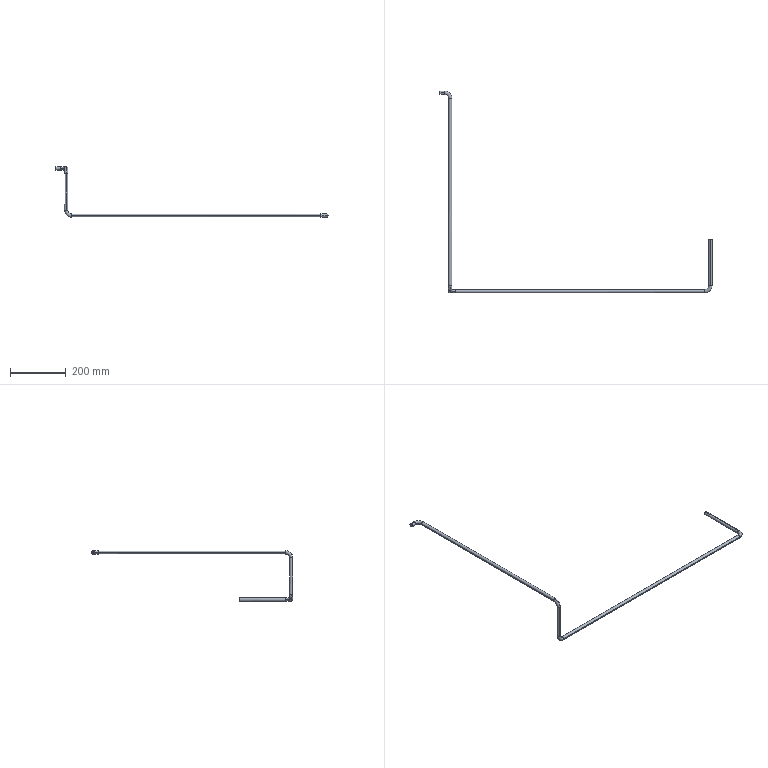Part | SolidWorks | features 3DProfileFeature 2, Sweep 1 | 1 solid | 38 faces | box 973.153 x 721.496 x 180.841 mm | volume 69029 mm3 | cylinder 20 | torus 16 | plane 2 | commonest cylinder face diameters 10 x10 12 x10
STEP:
#1=CARTESIAN_POINT('',(944.95,1782.095,424.913));
#2=VERTEX_POINT('',#1);
#3=CARTESIAN_POINT('',(954.95,1782.095,424.913));
#4=VERTEX_POINT('',#3);
#5=CARTESIAN_POINT('',(949.95,1782.095,424.913));
#6=DIRECTION('',(0.,-1.,0.));
#7=DIRECTION('',(0.,0.,-1.));
#8=AXIS2_PLACEMENT_3D('',#5,#6,#7);
#9=CIRCLE('',#8,5.);
#10=EDGE_CURVE('',#2,#4,#9,.T.);
#11=ORIENTED_EDGE('',*,*,#10,.T.);
#12=CARTESIAN_POINT('',(929.95,1807.095,424.913));
#13=VERTEX_POINT('',#12);
#14=CARTESIAN_POINT('',(929.95,1782.095,424.913));
#15=DIRECTION('',(0.,0.,1.));
#16=DIRECTION('',(1.,0.,0.));
#17=AXIS2_PLACEMENT_3D('',#14,#15,#16);
#18=CIRCLE('',#17,25.);
#19=EDGE_CURVE('',#4,#13,#18,.T.);
#20=ORIENTED_EDGE('',*,*,#19,.T.);
#21=CARTESIAN_POINT('',(929.95,1802.095,419.913));
#22=VERTEX_POINT('',#21);
#23=CARTESIAN_POINT('',(929.95,1802.095,424.913));
#24=DIRECTION('',(1.,0.,0.));
#25=DIRECTION('',(0.,0.,-1.));
#26=AXIS2_PLACEMENT_3D('',#23,#24,#25);
#27=CIRCLE('',#26,5.);
#28=EDGE_CURVE('',#22,#13,#27,.T.);
#29=ORIENTED_EDGE('',*,*,#28,.F.);
#30=CARTESIAN_POINT('',(929.95,1797.095,424.913));
#31=VERTEX_POINT('',#30);
#32=CARTESIAN_POINT('',(929.95,1802.095,424.913));
#33=DIRECTION('',(1.,0.,0.));
#34=DIRECTION('',(0.,0.,-1.));
#35=AXIS2_PLACEMENT_3D('',#32,#33,#34);
#36=CIRCLE('',#35,5.);
#37=EDGE_CURVE('',#31,#22,#36,.T.);
#38=ORIENTED_EDGE('',*,*,#37,.F.);
#39=CARTESIAN_POINT('',(929.95,1782.095,424.913));
#40=DIRECTION('',(0.,0.,1.));
#41=DIRECTION('',(1.,0.,0.));
#42=AXIS2_PLACEMENT_3D('',#39,#40,#41);
#43=CIRCLE('',#42,15.);
#44=EDGE_CURVE('',#2,#31,#43,.T.);
#45=ORIENTED_EDGE('',*,*,#44,.F.);
#46=EDGE_LOOP('',(#11,#20,#29,#38,#45));
#47=FACE_OUTER_BOUND('',#46,.T.);
#48=CARTESIAN_POINT('',(929.95,1782.095,424.913));
#49=DIRECTION('',(0.,0.,1.));
#50=DIRECTION('',(1.,0.,0.));
#51=AXIS2_PLACEMENT_3D('',#48,#49,#50);
#52=TOROIDAL_SURFACE('',#51,20.,5.);
#53=ADVANCED_FACE('',(#47),#52,.F.);
#54=CARTESIAN_POINT('',(949.95,1097.599,404.913));
#55=VERTEX_POINT('',#54);
#56=CARTESIAN_POINT('',(949.95,1087.599,404.913));
#57=VERTEX_POINT('',#56);
#58=CARTESIAN_POINT('',(949.95,1092.599,404.913));
#59=DIRECTION('',(0.,0.,-1.));
#60=DIRECTION('',(0.,1.,0.));
#61=AXIS2_PLACEMENT_3D('',#58,#59,#60);
#62=CIRCLE('',#61,5.);
#63=EDGE_CURVE('',#55,#57,#62,.T.);
#64=ORIENTED_EDGE('',*,*,#63,.T.);
#65=CARTESIAN_POINT('',(949.95,1112.599,429.913));
#66=VERTEX_POINT('',#65);
#67=CARTESIAN_POINT('',(949.95,1112.599,404.913));
#68=DIRECTION('',(-1.,0.,0.));
#69=DIRECTION('',(0.,0.,1.));
#70=AXIS2_PLACEMENT_3D('',#67,#68,#69);
#71=CIRCLE('',#70,25.);
#72=EDGE_CURVE('',#57,#66,#71,.T.);
#73=ORIENTED_EDGE('',*,*,#72,.T.);
#74=CARTESIAN_POINT('',(954.95,1112.599,424.913));
#75=VERTEX_POINT('',#74);
#76=CARTESIAN_POINT('',(949.95,1112.599,424.913));
#77=DIRECTION('',(0.,-1.,0.));
#78=DIRECTION('',(0.,0.,-1.));
#79=AXIS2_PLACEMENT_3D('',#76,#77,#78);
#80=CIRCLE('',#79,5.);
#81=EDGE_CURVE('',#75,#66,#80,.T.);
#82=ORIENTED_EDGE('',*,*,#81,.F.);
#83=CARTESIAN_POINT('',(949.95,1112.599,419.913));
#84=VERTEX_POINT('',#83);
#85=CARTESIAN_POINT('',(949.95,1112.599,424.913));
#86=DIRECTION('',(0.,-1.,0.));
#87=DIRECTION('',(0.,0.,-1.));
#88=AXIS2_PLACEMENT_3D('',#85,#86,#87);
#89=CIRCLE('',#88,5.);
#90=EDGE_CURVE('',#84,#75,#89,.T.);
#91=ORIENTED_EDGE('',*,*,#90,.F.);
#92=CARTESIAN_POINT('',(949.95,1112.599,404.913));
#93=DIRECTION('',(-1.,0.,0.));
#94=DIRECTION('',(0.,0.,1.));
#95=AXIS2_PLACEMENT_3D('',#92,#93,#94);
#96=CIRCLE('',#95,15.);
#97=EDGE_CURVE('',#55,#84,#96,.T.);
#98=ORIENTED_EDGE('',*,*,#97,.F.);
#99=EDGE_LOOP('',(#64,#73,#82,#91,#98));
#100=FACE_OUTER_BOUND('',#99,.T.);
#101=CARTESIAN_POINT('',(949.95,1112.599,404.913));
#102=DIRECTION('',(-1.,0.,0.));
#103=DIRECTION('',(0.,0.,1.));
#104=AXIS2_PLACEMENT_3D('',#101,#102,#103);
#105=TOROIDAL_SURFACE('',#104,20.,5.);
#106=ADVANCED_FACE('',(#100),#105,.F.);
#107=CARTESIAN_POINT('',(969.95,1087.599,256.072));
#108=VERTEX_POINT('',#107);
#109=CARTESIAN_POINT('',(969.95,1092.599,251.072));
#110=VERTEX_POINT('',#109);
#111=CARTESIAN_POINT('',(969.95,1092.599,256.072));
#112=DIRECTION('',(1.,0.,0.));
#113=DIRECTION('',(0.,1.,0.));
#114=AXIS2_PLACEMENT_3D('',#111,#112,#113);
#115=CIRCLE('',#114,5.);
#116=EDGE_CURVE('',#108,#110,#115,.T.);
#117=ORIENTED_EDGE('',*,*,#116,.T.);
#118=CARTESIAN_POINT('',(944.95,1092.599,276.072));
#119=VERTEX_POINT('',#118);
#120=CARTESIAN_POINT('',(969.95,1092.599,276.072));
#121=DIRECTION('',(0.,1.,0.));
#122=DIRECTION('',(-1.,0.,0.));
#123=AXIS2_PLACEMENT_3D('',#120,#121,#122);
#124=CIRCLE('',#123,25.);
#125=EDGE_CURVE('',#110,#119,#124,.T.);
#126=ORIENTED_EDGE('',*,*,#125,.T.);
#127=CARTESIAN_POINT('',(949.95,1087.599,276.072));
#128=VERTEX_POINT('',#127);
#129=CARTESIAN_POINT('',(949.95,1092.599,276.072));
#130=DIRECTION('',(0.,0.,-1.));
#131=DIRECTION('',(0.,1.,0.));
#132=AXIS2_PLACEMENT_3D('',#129,#130,#131);
#133=CIRCLE('',#132,5.);
#134=EDGE_CURVE('',#128,#119,#133,.T.);
#135=ORIENTED_EDGE('',*,*,#134,.F.);
#136=CARTESIAN_POINT('',(954.95,1092.599,276.072));
#137=VERTEX_POINT('',#136);
#138=CARTESIAN_POINT('',(949.95,1092.599,276.072));
#139=DIRECTION('',(0.,0.,-1.));
#140=DIRECTION('',(0.,1.,0.));
#141=AXIS2_PLACEMENT_3D('',#138,#139,#140);
#142=CIRCLE('',#141,5.);
#143=EDGE_CURVE('',#137,#128,#142,.T.);
#144=ORIENTED_EDGE('',*,*,#143,.F.);
#145=CARTESIAN_POINT('',(969.95,1092.599,261.072));
#146=VERTEX_POINT('',#145);
#147=CARTESIAN_POINT('',(969.95,1092.599,276.072));
#148=DIRECTION('',(0.,1.,0.));
#149=DIRECTION('',(-1.,0.,0.));
#150=AXIS2_PLACEMENT_3D('',#147,#148,#149);
#151=CIRCLE('',#150,15.);
#152=EDGE_CURVE('',#146,#137,#151,.T.);
#153=ORIENTED_EDGE('',*,*,#152,.F.);
#154=CARTESIAN_POINT('',(969.95,1092.599,256.072));
#155=DIRECTION('',(1.,0.,0.));
#156=DIRECTION('',(0.,1.,0.));
#157=AXIS2_PLACEMENT_3D('',#154,#155,#156);
#158=CIRCLE('',#157,5.);
#159=EDGE_CURVE('',#146,#108,#158,.T.);
#160=ORIENTED_EDGE('',*,*,#159,.T.);
#161=EDGE_LOOP('',(#117,#126,#135,#144,#153,#160));
#162=FACE_OUTER_BOUND('',#161,.T.);
#163=CARTESIAN_POINT('',(969.95,1092.599,276.072));
#164=DIRECTION('',(0.,1.,0.));
#165=DIRECTION('',(-1.,0.,0.));
#166=AXIS2_PLACEMENT_3D('',#163,#164,#165);
#167=TOROIDAL_SURFACE('',#166,20.,5.);
#168=ADVANCED_FACE('',(#162),#167,.F.);
#169=CARTESIAN_POINT('',(1880.513,1112.599,261.072));
#170=VERTEX_POINT('',#169);
#171=CARTESIAN_POINT('',(1885.513,1112.599,256.072));
#172=VERTEX_POINT('',#171);
#173=CARTESIAN_POINT('',(1880.513,1112.599,256.072));
#174=DIRECTION('',(0.,1.,0.));
#175=DIRECTION('',(-1.,0.,0.));
#176=AXIS2_PLACEMENT_3D('',#173,#174,#175);
#177=CIRCLE('',#176,5.);
#178=EDGE_CURVE('',#170,#172,#177,.T.);
#179=ORIENTED_EDGE('',*,*,#178,.T.);
#180=CARTESIAN_POINT('',(1860.513,1087.599,256.072));
#181=VERTEX_POINT('',#180);
#182=CARTESIAN_POINT('',(1860.513,1112.599,256.072));
#183=DIRECTION('',(0.,0.,-1.));
#184=DIRECTION('',(-1.,0.,0.));
#185=AXIS2_PLACEMENT_3D('',#182,#183,#184);
#186=CIRCLE('',#185,25.);
#187=EDGE_CURVE('',#172,#181,#186,.T.);
#188=ORIENTED_EDGE('',*,*,#187,.T.);
#189=CARTESIAN_POINT('',(1860.513,1097.599,256.072));
#190=VERTEX_POINT('',#189);
#191=CARTESIAN_POINT('',(1860.513,1092.599,256.072));
#192=DIRECTION('',(1.,0.,0.));
#193=DIRECTION('',(0.,1.,0.));
#194=AXIS2_PLACEMENT_3D('',#191,#192,#193);
#195=CIRCLE('',#194,5.);
#196=EDGE_CURVE('',#190,#181,#195,.T.);
#197=ORIENTED_EDGE('',*,*,#196,.F.);
#198=CARTESIAN_POINT('',(1875.513,1112.599,256.072));
#199=VERTEX_POINT('',#198);
#200=CARTESIAN_POINT('',(1860.513,1112.599,256.072));
#201=DIRECTION('',(0.,0.,-1.));
#202=DIRECTION('',(-1.,0.,0.));
#203=AXIS2_PLACEMENT_3D('',#200,#201,#202);
#204=CIRCLE('',#203,15.);
#205=EDGE_CURVE('',#199,#190,#204,.T.);
#206=ORIENTED_EDGE('',*,*,#205,.F.);
#207=CARTESIAN_POINT('',(1880.513,1112.599,256.072));
#208=DIRECTION('',(0.,1.,0.));
#209=DIRECTION('',(-1.,0.,0.));
#210=AXIS2_PLACEMENT_3D('',#207,#208,#209);
#211=CIRCLE('',#210,5.);
#212=EDGE_CURVE('',#199,#170,#211,.T.);
#213=ORIENTED_EDGE('',*,*,#212,.T.);
#214=EDGE_LOOP('',(#179,#188,#197,#206,#213));
#215=FACE_OUTER_BOUND('',#214,.T.);
#216=CARTESIAN_POINT('',(1860.513,1112.599,256.072));
#217=DIRECTION('',(0.,0.,-1.));
#218=DIRECTION('',(-1.,0.,0.));
#219=AXIS2_PLACEMENT_3D('',#216,#217,#218);
#220=TOROIDAL_SURFACE('',#219,20.,5.);
#221=ADVANCED_FACE('',(#215),#220,.F.);
#222=CARTESIAN_POINT('',(955.95,1782.095,424.913));
#223=VERTEX_POINT('',#222);
#224=CARTESIAN_POINT('',(943.95,1782.095,424.913));
#225=VERTEX_POINT('',#224);
#226=CARTESIAN_POINT('',(949.95,1782.095,424.913));
#227=DIRECTION('',(0.,-1.,0.));
#228=DIRECTION('',(-1.,0.,0.));
#229=AXIS2_PLACEMENT_3D('',#226,#227,#228);
#230=CIRCLE('',#229,6.);
#231=EDGE_CURVE('',#223,#225,#230,.T.);
#232=ORIENTED_EDGE('',*,*,#231,.F.);
#233=CARTESIAN_POINT('',(929.95,1808.095,424.913));
#234=VERTEX_POINT('',#233);
#235=CARTESIAN_POINT('',(929.95,1782.095,424.913));
#236=DIRECTION('',(0.,0.,1.));
#237=DIRECTION('',(1.,0.,0.));
#238=AXIS2_PLACEMENT_3D('',#235,#236,#237);
#239=CIRCLE('',#238,26.);
#240=EDGE_CURVE('',#223,#234,#239,.T.);
#241=ORIENTED_EDGE('',*,*,#240,.T.);
#242=CARTESIAN_POINT('',(929.95,1802.095,430.913));
#243=VERTEX_POINT('',#242);
#244=CARTESIAN_POINT('',(929.95,1802.095,424.913));
#245=DIRECTION('',(1.,0.,0.));
#246=DIRECTION('',(0.,1.,0.));
#247=AXIS2_PLACEMENT_3D('',#244,#245,#246);
#248=CIRCLE('',#247,6.);
#249=EDGE_CURVE('',#234,#243,#248,.T.);
#250=ORIENTED_EDGE('',*,*,#249,.T.);
#251=CARTESIAN_POINT('',(929.95,1796.095,424.913));
#252=VERTEX_POINT('',#251);
#253=CARTESIAN_POINT('',(929.95,1802.095,424.913));
#254=DIRECTION('',(1.,0.,0.));
#255=DIRECTION('',(0.,1.,0.));
#256=AXIS2_PLACEMENT_3D('',#253,#254,#255);
#257=CIRCLE('',#256,6.);
#258=EDGE_CURVE('',#243,#252,#257,.T.);
#259=ORIENTED_EDGE('',*,*,#258,.T.);
#260=CARTESIAN_POINT('',(929.95,1782.095,424.913));
#261=DIRECTION('',(0.,0.,1.));
#262=DIRECTION('',(1.,0.,0.));
#263=AXIS2_PLACEMENT_3D('',#260,#261,#262);
#264=CIRCLE('',#263,14.);
#265=EDGE_CURVE('',#225,#252,#264,.T.);
#266=ORIENTED_EDGE('',*,*,#265,.F.);
#267=EDGE_LOOP('',(#232,#241,#250,#259,#266));
#268=FACE_OUTER_BOUND('',#267,.T.);
#269=CARTESIAN_POINT('',(929.95,1782.095,424.913));
#270=DIRECTION('',(0.,0.,1.));
#271=DIRECTION('',(1.,0.,0.));
#272=AXIS2_PLACEMENT_3D('',#269,#270,#271);
#273=TOROIDAL_SURFACE('',#272,20.,6.);
#274=ADVANCED_FACE('',(#268),#273,.T.);
#275=CARTESIAN_POINT('',(949.95,1086.599,404.913));
#276=VERTEX_POINT('',#275);
#277=CARTESIAN_POINT('',(949.95,1098.599,404.913));
#278=VERTEX_POINT('',#277);
#279=CARTESIAN_POINT('',(949.95,1092.599,404.913));
#280=DIRECTION('',(0.,0.,-1.));
#281=DIRECTION('',(0.,-1.,0.));
#282=AXIS2_PLACEMENT_3D('',#279,#280,#281);
#283=CIRCLE('',#282,6.);
#284=EDGE_CURVE('',#276,#278,#283,.T.);
#285=ORIENTED_EDGE('',*,*,#284,.F.);
#286=CARTESIAN_POINT('',(949.95,1112.599,430.913));
#287=VERTEX_POINT('',#286);
#288=CARTESIAN_POINT('',(949.95,1112.599,404.913));
#289=DIRECTION('',(-1.,0.,0.));
#290=DIRECTION('',(0.,0.,1.));
#291=AXIS2_PLACEMENT_3D('',#288,#289,#290);
#292=CIRCLE('',#291,26.);
#293=EDGE_CURVE('',#276,#287,#292,.T.);
#294=ORIENTED_EDGE('',*,*,#293,.T.);
#295=CARTESIAN_POINT('',(943.95,1112.599,424.913));
#296=VERTEX_POINT('',#295);
#297=CARTESIAN_POINT('',(949.95,1112.599,424.913));
#298=DIRECTION('',(0.,-1.,0.));
#299=DIRECTION('',(0.,0.,-1.));
#300=AXIS2_PLACEMENT_3D('',#297,#298,#299);
#301=CIRCLE('',#300,6.);
#302=EDGE_CURVE('',#287,#296,#301,.T.);
#303=ORIENTED_EDGE('',*,*,#302,.T.);
#304=CARTESIAN_POINT('',(949.95,1112.599,418.913));
#305=VERTEX_POINT('',#304);
#306=CARTESIAN_POINT('',(949.95,1112.599,424.913));
#307=DIRECTION('',(0.,-1.,0.));
#308=DIRECTION('',(0.,0.,-1.));
#309=AXIS2_PLACEMENT_3D('',#306,#307,#308);
#310=CIRCLE('',#309,6.);
#311=EDGE_CURVE('',#296,#305,#310,.T.);
#312=ORIENTED_EDGE('',*,*,#311,.T.);
#313=CARTESIAN_POINT('',(949.95,1112.599,404.913));
#314=DIRECTION('',(-1.,0.,0.));
#315=DIRECTION('',(0.,0.,1.));
#316=AXIS2_PLACEMENT_3D('',#313,#314,#315);
#317=CIRCLE('',#316,14.);
#318=EDGE_CURVE('',#278,#305,#317,.T.);
#319=ORIENTED_EDGE('',*,*,#318,.F.);
#320=EDGE_LOOP('',(#285,#294,#303,#312,#319));
#321=FACE_OUTER_BOUND('',#320,.T.);
#322=CARTESIAN_POINT('',(949.95,1112.599,404.913));
#323=DIRECTION('',(-1.,0.,0.));
#324=DIRECTION('',(0.,0.,1.));
#325=AXIS2_PLACEMENT_3D('',#322,#323,#324);
#326=TOROIDAL_SURFACE('',#325,20.,6.);
#327=ADVANCED_FACE('',(#321),#326,.T.);
#328=CARTESIAN_POINT('',(969.95,1092.599,250.072));
#329=VERTEX_POINT('',#328);
#330=CARTESIAN_POINT('',(969.95,1098.599,256.072));
#331=VERTEX_POINT('',#330);
#332=CARTESIAN_POINT('',(969.95,1092.599,256.072));
#333=DIRECTION('',(1.,0.,0.));
#334=DIRECTION('',(0.,-1.,0.));
#335=AXIS2_PLACEMENT_3D('',#332,#333,#334);
#336=CIRCLE('',#335,6.);
#337=EDGE_CURVE('',#329,#331,#336,.T.);
#338=ORIENTED_EDGE('',*,*,#337,.F.);
#339=CARTESIAN_POINT('',(943.95,1092.599,276.072));
#340=VERTEX_POINT('',#339);
#341=CARTESIAN_POINT('',(969.95,1092.599,276.072));
#342=DIRECTION('',(0.,1.,0.));
#343=DIRECTION('',(-1.,0.,0.));
#344=AXIS2_PLACEMENT_3D('',#341,#342,#343);
#345=CIRCLE('',#344,26.);
#346=EDGE_CURVE('',#329,#340,#345,.T.);
#347=ORIENTED_EDGE('',*,*,#346,.T.);
#348=CARTESIAN_POINT('',(949.95,1098.599,276.072));
#349=VERTEX_POINT('',#348);
#350=CARTESIAN_POINT('',(949.95,1092.599,276.072));
#351=DIRECTION('',(0.,0.,-1.));
#352=DIRECTION('',(-1.,0.,0.));
#353=AXIS2_PLACEMENT_3D('',#350,#351,#352);
#354=CIRCLE('',#353,6.);
#355=EDGE_CURVE('',#340,#349,#354,.T.);
#356=ORIENTED_EDGE('',*,*,#355,.T.);
#357=CARTESIAN_POINT('',(955.95,1092.599,276.072));
#358=VERTEX_POINT('',#357);
#359=CARTESIAN_POINT('',(949.95,1092.599,276.072));
#360=DIRECTION('',(0.,0.,-1.));
#361=DIRECTION('',(-1.,0.,0.));
#362=AXIS2_PLACEMENT_3D('',#359,#360,#361);
#363=CIRCLE('',#362,6.);
#364=EDGE_CURVE('',#349,#358,#363,.T.);
#365=ORIENTED_EDGE('',*,*,#364,.T.);
#366=CARTESIAN_POINT('',(969.95,1092.599,262.072));
#367=VERTEX_POINT('',#366);
#368=CARTESIAN_POINT('',(969.95,1092.599,276.072));
#369=DIRECTION('',(0.,1.,0.));
#370=DIRECTION('',(-1.,0.,0.));
#371=AXIS2_PLACEMENT_3D('',#368,#369,#370);
#372=CIRCLE('',#371,14.);
#373=EDGE_CURVE('',#367,#358,#372,.T.);
#374=ORIENTED_EDGE('',*,*,#373,.F.);
#375=CARTESIAN_POINT('',(969.95,1092.599,256.072));
#376=DIRECTION('',(1.,0.,0.));
#377=DIRECTION('',(0.,-1.,0.));
#378=AXIS2_PLACEMENT_3D('',#375,#376,#377);
#379=CIRCLE('',#378,6.);
#380=EDGE_CURVE('',#331,#367,#379,.T.);
#381=ORIENTED_EDGE('',*,*,#380,.F.);
#382=EDGE_LOOP('',(#338,#347,#356,#365,#374,#381));
#383=FACE_OUTER_BOUND('',#382,.T.);
#384=CARTESIAN_POINT('',(969.95,1092.599,276.072));
#385=DIRECTION('',(0.,1.,0.));
#386=DIRECTION('',(-1.,0.,0.));
#387=AXIS2_PLACEMENT_3D('',#384,#385,#386);
#388=TOROIDAL_SURFACE('',#387,20.,6.);
#389=ADVANCED_FACE('',(#383),#388,.T.);
#390=CARTESIAN_POINT('',(1886.513,1112.599,256.072));
#391=VERTEX_POINT('',#390);
#392=CARTESIAN_POINT('',(1880.513,1112.599,250.072));
#393=VERTEX_POINT('',#392);
#394=CARTESIAN_POINT('',(1880.513,1112.599,256.072));
#395=DIRECTION('',(0.,1.,0.));
#396=DIRECTION('',(0.,0.,-1.));
#397=AXIS2_PLACEMENT_3D('',#394,#395,#396);
#398=CIRCLE('',#397,6.);
#399=EDGE_CURVE('',#391,#393,#398,.T.);
#400=ORIENTED_EDGE('',*,*,#399,.F.);
#401=CARTESIAN_POINT('',(1860.513,1086.599,256.072));
#402=VERTEX_POINT('',#401);
#403=CARTESIAN_POINT('',(1860.513,1112.599,256.072));
#404=DIRECTION('',(0.,0.,-1.));
#405=DIRECTION('',(-1.,0.,0.));
#406=AXIS2_PLACEMENT_3D('',#403,#404,#405);
#407=CIRCLE('',#406,26.);
#408=EDGE_CURVE('',#391,#402,#407,.T.);
#409=ORIENTED_EDGE('',*,*,#408,.T.);
#410=CARTESIAN_POINT('',(1860.513,1098.599,256.072));
#411=VERTEX_POINT('',#410);
#412=CARTESIAN_POINT('',(1860.513,1092.599,256.072));
#413=DIRECTION('',(1.,0.,0.));
#414=DIRECTION('',(0.,1.,0.));
#415=AXIS2_PLACEMENT_3D('',#412,#413,#414);
#416=CIRCLE('',#415,6.);
#417=EDGE_CURVE('',#402,#411,#416,.T.);
#418=ORIENTED_EDGE('',*,*,#417,.T.);
#419=CARTESIAN_POINT('',(1874.513,1112.599,256.072));
#420=VERTEX_POINT('',#419);
#421=CARTESIAN_POINT('',(1860.513,1112.599,256.072));
#422=DIRECTION('',(0.,0.,-1.));
#423=DIRECTION('',(-1.,0.,0.));
#424=AXIS2_PLACEMENT_3D('',#421,#422,#423);
#425=CIRCLE('',#424,14.);
#426=EDGE_CURVE('',#420,#411,#425,.T.);
#427=ORIENTED_EDGE('',*,*,#426,.F.);
#428=CARTESIAN_POINT('',(1880.513,1112.599,256.072));
#429=DIRECTION('',(0.,1.,0.));
#430=DIRECTION('',(0.,0.,-1.));
#431=AXIS2_PLACEMENT_3D('',#428,#429,#430);
#432=CIRCLE('',#431,6.);
#433=EDGE_CURVE('',#393,#420,#432,.T.);
#434=ORIENTED_EDGE('',*,*,#433,.F.);
#435=EDGE_LOOP('',(#400,#409,#418,#427,#434));
#436=FACE_OUTER_BOUND('',#435,.T.);
#437=CARTESIAN_POINT('',(1860.513,1112.599,256.072));
#438=DIRECTION('',(0.,0.,-1.));
#439=DIRECTION('',(-1.,0.,0.));
#440=AXIS2_PLACEMENT_3D('',#437,#438,#439);
#441=TOROIDAL_SURFACE('',#440,20.,6.);
#442=ADVANCED_FACE('',(#436),#441,.T.);
#443=CARTESIAN_POINT('',(929.95,1802.095,429.913));
#444=VERTEX_POINT('',#443);
#445=CARTESIAN_POINT('',(929.95,1802.095,424.913));
#446=DIRECTION('',(1.,0.,0.));
#447=DIRECTION('',(0.,0.,-1.));
#448=AXIS2_PLACEMENT_3D('',#445,#446,#447);
#449=CIRCLE('',#448,5.);
#450=EDGE_CURVE('',#444,#31,#449,.T.);
#451=ORIENTED_EDGE('',*,*,#450,.T.);
#452=ORIENTED_EDGE('',*,*,#37,.T.);
#453=CARTESIAN_POINT('',(913.359,1802.095,419.913));
#454=VERTEX_POINT('',#453);
#455=CARTESIAN_POINT('',(929.95,1802.095,419.913));
#456=DIRECTION('',(-1.,0.,0.));
#457=VECTOR('',#456,1000.);
#458=LINE('',#455,#457);
#459=EDGE_CURVE('',#22,#454,#458,.T.);
#460=ORIENTED_EDGE('',*,*,#459,.T.);
#461=CARTESIAN_POINT('',(913.359,1802.095,429.913));
#462=VERTEX_POINT('',#461);
#463=CARTESIAN_POINT('',(913.359,1802.095,424.913));
#464=DIRECTION('',(1.,0.,0.));
#465=DIRECTION('',(0.,0.,-1.));
#466=AXIS2_PLACEMENT_3D('',#463,#464,#465);
#467=CIRCLE('',#466,5.);
#468=EDGE_CURVE('',#462,#454,#467,.T.);
#469=ORIENTED_EDGE('',*,*,#468,.F.);
#470=CARTESIAN_POINT('',(929.95,1802.095,429.913));
#471=DIRECTION('',(-1.,0.,0.));
#472=VECTOR('',#471,1000.);
#473=LINE('',#470,#472);
#474=EDGE_CURVE('',#444,#462,#473,.T.);
#475=ORIENTED_EDGE('',*,*,#474,.F.);
#476=EDGE_LOOP('',(#451,#452,#460,#469,#475));
#477=FACE_OUTER_BOUND('',#476,.T.);
#478=CARTESIAN_POINT('',(929.95,1802.095,424.913));
#479=DIRECTION('',(-1.,0.,0.));
#480=DIRECTION('',(0.,0.,1.));
#481=AXIS2_PLACEMENT_3D('',#478,#479,#480);
#482=CYLINDRICAL_SURFACE('',#481,5.);
#483=ADVANCED_FACE('',(#477),#482,.F.);
#484=CARTESIAN_POINT('',(944.95,1112.599,424.913));
#485=VERTEX_POINT('',#484);
#486=CARTESIAN_POINT('',(949.95,1112.599,424.913));
#487=DIRECTION('',(0.,-1.,0.));
#488=DIRECTION('',(0.,0.,-1.));
#489=AXIS2_PLACEMENT_3D('',#486,#487,#488);
#490=CIRCLE('',#489,5.);
#491=EDGE_CURVE('',#485,#84,#490,.T.);
#492=ORIENTED_EDGE('',*,*,#491,.T.);
#493=ORIENTED_EDGE('',*,*,#90,.T.);
#494=CARTESIAN_POINT('',(954.95,1112.599,424.913));
#495=DIRECTION('',(0.,1.,0.));
#496=VECTOR('',#495,1000.);
#497=LINE('',#494,#496);
#498=EDGE_CURVE('',#75,#4,#497,.T.);
#499=ORIENTED_EDGE('',*,*,#498,.T.);
#500=ORIENTED_EDGE('',*,*,#10,.F.);
#501=CARTESIAN_POINT('',(944.95,1112.599,424.913));
#502=DIRECTION('',(0.,1.,0.));
#503=VECTOR('',#502,1000.);
#504=LINE('',#501,#503);
#505=EDGE_CURVE('',#485,#2,#504,.T.);
#506=ORIENTED_EDGE('',*,*,#505,.F.);
#507=EDGE_LOOP('',(#492,#493,#499,#500,#506));
#508=FACE_OUTER_BOUND('',#507,.T.);
#509=CARTESIAN_POINT('',(949.95,1112.599,424.913));
#510=DIRECTION('',(0.,1.,0.));
#511=DIRECTION('',(-1.,0.,0.));
#512=AXIS2_PLACEMENT_3D('',#509,#510,#511);
#513=CYLINDRICAL_SURFACE('',#512,5.);
#514=ADVANCED_FACE('',(#508),#513,.F.);
#515=ORIENTED_EDGE('',*,*,#134,.T.);
#516=CARTESIAN_POINT('',(949.95,1097.599,276.072));
#517=VERTEX_POINT('',#516);
#518=CARTESIAN_POINT('',(949.95,1092.599,276.072));
#519=DIRECTION('',(0.,0.,-1.));
#520=DIRECTION('',(0.,1.,0.));
#521=AXIS2_PLACEMENT_3D('',#518,#519,#520);
#522=CIRCLE('',#521,5.);
#523=EDGE_CURVE('',#119,#517,#522,.T.);
#524=ORIENTED_EDGE('',*,*,#523,.T.);
#525=CARTESIAN_POINT('',(949.95,1097.599,276.072));
#526=DIRECTION('',(0.,0.,1.));
#527=VECTOR('',#526,1000.);
#528=LINE('',#525,#527);
#529=EDGE_CURVE('',#517,#55,#528,.T.);
#530=ORIENTED_EDGE('',*,*,#529,.T.);
#531=CARTESIAN_POINT('',(949.95,1092.599,404.913));
#532=DIRECTION('',(0.,0.,-1.));
#533=DIRECTION('',(0.,1.,0.));
#534=AXIS2_PLACEMENT_3D('',#531,#532,#533);
#535=CIRCLE('',#534,5.);
#536=EDGE_CURVE('',#57,#55,#535,.T.);
#537=ORIENTED_EDGE('',*,*,#536,.F.);
#538=CARTESIAN_POINT('',(949.95,1087.599,276.072));
#539=DIRECTION('',(0.,0.,1.));
#540=VECTOR('',#539,1000.);
#541=LINE('',#538,#540);
#542=EDGE_CURVE('',#128,#57,#541,.T.);
#543=ORIENTED_EDGE('',*,*,#542,.F.);
#544=EDGE_LOOP('',(#515,#524,#530,#537,#543));
#545=FACE_OUTER_BOUND('',#544,.T.);
#546=CARTESIAN_POINT('',(949.95,1092.599,276.072));
#547=DIRECTION('',(0.,0.,1.));
#548=DIRECTION('',(0.,-1.,0.));
#549=AXIS2_PLACEMENT_3D('',#546,#547,#548);
#550=CYLINDRICAL_SURFACE('',#549,5.);
#551=ADVANCED_FACE('',(#545),#550,.F.);
#552=CARTESIAN_POINT('',(1860.513,1092.599,256.072));
#553=DIRECTION('',(1.,0.,0.));
#554=DIRECTION('',(0.,1.,0.));
#555=AXIS2_PLACEMENT_3D('',#552,#553,#554);
#556=CIRCLE('',#555,5.);
#557=EDGE_CURVE('',#181,#190,#556,.T.);
#558=ORIENTED_EDGE('',*,*,#557,.T.);
#559=CARTESIAN_POINT('',(969.95,1097.599,256.072));
#560=VERTEX_POINT('',#559);
#561=CARTESIAN_POINT('',(1860.513,1097.599,256.072));
#562=DIRECTION('',(-1.,0.,0.));
#563=VECTOR('',#562,1000.);
#564=LINE('',#561,#563);
#565=EDGE_CURVE('',#190,#560,#564,.T.);
#566=ORIENTED_EDGE('',*,*,#565,.T.);
#567=CARTESIAN_POINT('',(969.95,1092.599,256.072));
#568=DIRECTION('',(1.,0.,0.));
#569=DIRECTION('',(0.,1.,0.));
#570=AXIS2_PLACEMENT_3D('',#567,#568,#569);
#571=CIRCLE('',#570,5.);
#572=EDGE_CURVE('',#110,#560,#571,.T.);
#573=ORIENTED_EDGE('',*,*,#572,.F.);
#574=ORIENTED_EDGE('',*,*,#116,.F.);
#575=CARTESIAN_POINT('',(1860.513,1087.599,256.072));
#576=DIRECTION('',(-1.,0.,0.));
#577=VECTOR('',#576,1000.);
#578=LINE('',#575,#577);
#579=EDGE_CURVE('',#181,#108,#578,.T.);
#580=ORIENTED_EDGE('',*,*,#579,.F.);
#581=EDGE_LOOP('',(#558,#566,#573,#574,#580));
#582=FACE_OUTER_BOUND('',#581,.T.);
#583=CARTESIAN_POINT('',(1860.513,1092.599,256.072));
#584=DIRECTION('',(-1.,0.,0.));
#585=DIRECTION('',(0.,-1.,0.));
#586=AXIS2_PLACEMENT_3D('',#583,#584,#585);
#587=CYLINDRICAL_SURFACE('',#586,5.);
#588=ADVANCED_FACE('',(#582),#587,.F.);
#589=CARTESIAN_POINT('',(1880.513,1278.953,251.072));
#590=VERTEX_POINT('',#589);
#591=CARTESIAN_POINT('',(1880.513,1278.953,261.072));
#592=VERTEX_POINT('',#591);
#593=CARTESIAN_POINT('',(1880.513,1278.953,256.072));
#594=DIRECTION('',(0.,1.,0.));
#595=DIRECTION('',(-1.,0.,0.));
#596=AXIS2_PLACEMENT_3D('',#593,#594,#595);
#597=CIRCLE('',#596,5.);
#598=EDGE_CURVE('',#590,#592,#597,.T.);
#599=ORIENTED_EDGE('',*,*,#598,.T.);
#600=CARTESIAN_POINT('',(1880.513,1278.953,261.072));
#601=DIRECTION('',(0.,-1.,0.));
#602=VECTOR('',#601,1000.);
#603=LINE('',#600,#602);
#604=EDGE_CURVE('',#592,#170,#603,.T.);
#605=ORIENTED_EDGE('',*,*,#604,.T.);
#606=ORIENTED_EDGE('',*,*,#212,.F.);
#607=CARTESIAN_POINT('',(1880.513,1112.599,251.072));
#608=VERTEX_POINT('',#607);
#609=CARTESIAN_POINT('',(1880.513,1112.599,256.072));
#610=DIRECTION('',(0.,1.,0.));
#611=DIRECTION('',(-1.,0.,0.));
#612=AXIS2_PLACEMENT_3D('',#609,#610,#611);
#613=CIRCLE('',#612,5.);
#614=EDGE_CURVE('',#608,#199,#613,.T.);
#615=ORIENTED_EDGE('',*,*,#614,.F.);
#616=CARTESIAN_POINT('',(1880.513,1278.953,251.072));
#617=DIRECTION('',(0.,-1.,0.));
#618=VECTOR('',#617,1000.);
#619=LINE('',#616,#618);
#620=EDGE_CURVE('',#590,#608,#619,.T.);
#621=ORIENTED_EDGE('',*,*,#620,.F.);
#622=EDGE_LOOP('',(#599,#605,#606,#615,#621));
#623=FACE_OUTER_BOUND('',#622,.T.);
#624=CARTESIAN_POINT('',(1880.513,1278.953,256.072));
#625=DIRECTION('',(0.,-1.,0.));
#626=DIRECTION('',(0.,0.,-1.));
#627=AXIS2_PLACEMENT_3D('',#624,#625,#626);
#628=CYLINDRICAL_SURFACE('',#627,5.);
#629=ADVANCED_FACE('',(#623),#628,.F.);
#630=CARTESIAN_POINT('',(929.95,1802.095,418.913));
#631=VERTEX_POINT('',#630);
#632=CARTESIAN_POINT('',(929.95,1802.095,424.913));
#633=DIRECTION('',(1.,0.,0.));
#634=DIRECTION('',(0.,1.,0.));
#635=AXIS2_PLACEMENT_3D('',#632,#633,#634);
#636=CIRCLE('',#635,6.);
#637=EDGE_CURVE('',#631,#234,#636,.T.);
#638=ORIENTED_EDGE('',*,*,#637,.F.);
#639=CARTESIAN_POINT('',(913.359,1802.095,418.913));
#640=VERTEX_POINT('',#639);
#641=CARTESIAN_POINT('',(929.95,1802.095,418.913));
#642=DIRECTION('',(-1.,0.,0.));
#643=VECTOR('',#642,1000.);
#644=LINE('',#641,#643);
#645=EDGE_CURVE('',#631,#640,#644,.T.);
#646=ORIENTED_EDGE('',*,*,#645,.T.);
#647=CARTESIAN_POINT('',(913.359,1802.095,430.913));
#648=VERTEX_POINT('',#647);
#649=CARTESIAN_POINT('',(913.359,1802.095,424.913));
#650=DIRECTION('',(1.,0.,0.));
#651=DIRECTION('',(0.,0.,-1.));
#652=AXIS2_PLACEMENT_3D('',#649,#650,#651);
#653=CIRCLE('',#652,6.);
#654=EDGE_CURVE('',#640,#648,#653,.T.);
#655=ORIENTED_EDGE('',*,*,#654,.T.);
#656=CARTESIAN_POINT('',(929.95,1802.095,430.913));
#657=DIRECTION('',(-1.,0.,0.));
#658=VECTOR('',#657,1000.);
#659=LINE('',#656,#658);
#660=EDGE_CURVE('',#243,#648,#659,.T.);
#661=ORIENTED_EDGE('',*,*,#660,.F.);
#662=ORIENTED_EDGE('',*,*,#249,.F.);
#663=EDGE_LOOP('',(#638,#646,#655,#661,#662));
#664=FACE_OUTER_BOUND('',#663,.T.);
#665=CARTESIAN_POINT('',(929.95,1802.095,424.913));
#666=DIRECTION('',(-1.,0.,0.));
#667=DIRECTION('',(0.,0.,1.));
#668=AXIS2_PLACEMENT_3D('',#665,#666,#667);
#669=CYLINDRICAL_SURFACE('',#668,6.);
#670=ADVANCED_FACE('',(#664),#669,.T.);
#671=CARTESIAN_POINT('',(955.95,1112.599,424.913));
#672=VERTEX_POINT('',#671);
#673=CARTESIAN_POINT('',(949.95,1112.599,424.913));
#674=DIRECTION('',(0.,-1.,0.));
#675=DIRECTION('',(0.,0.,-1.));
#676=AXIS2_PLACEMENT_3D('',#673,#674,#675);
#677=CIRCLE('',#676,6.);
#678=EDGE_CURVE('',#672,#287,#677,.T.);
#679=ORIENTED_EDGE('',*,*,#678,.F.);
#680=CARTESIAN_POINT('',(955.95,1112.599,424.913));
#681=DIRECTION('',(0.,1.,0.));
#682=VECTOR('',#681,1000.);
#683=LINE('',#680,#682);
#684=EDGE_CURVE('',#672,#223,#683,.T.);
#685=ORIENTED_EDGE('',*,*,#684,.T.);
#686=ORIENTED_EDGE('',*,*,#231,.T.);
#687=CARTESIAN_POINT('',(943.95,1112.599,424.913));
#688=DIRECTION('',(0.,1.,0.));
#689=VECTOR('',#688,1000.);
#690=LINE('',#687,#689);
#691=EDGE_CURVE('',#296,#225,#690,.T.);
#692=ORIENTED_EDGE('',*,*,#691,.F.);
#693=ORIENTED_EDGE('',*,*,#302,.F.);
#694=EDGE_LOOP('',(#679,#685,#686,#692,#693));
#695=FACE_OUTER_BOUND('',#694,.T.);
#696=CARTESIAN_POINT('',(949.95,1112.599,424.913));
#697=DIRECTION('',(0.,1.,0.));
#698=DIRECTION('',(-1.,0.,0.));
#699=AXIS2_PLACEMENT_3D('',#696,#697,#698);
#700=CYLINDRICAL_SURFACE('',#699,6.);
#701=ADVANCED_FACE('',(#695),#700,.T.);
#702=ORIENTED_EDGE('',*,*,#364,.F.);
#703=CARTESIAN_POINT('',(949.95,1098.599,276.072));
#704=DIRECTION('',(0.,0.,1.));
#705=VECTOR('',#704,1000.);
#706=LINE('',#703,#705);
#707=EDGE_CURVE('',#349,#278,#706,.T.);
#708=ORIENTED_EDGE('',*,*,#707,.T.);
#709=CARTESIAN_POINT('',(949.95,1092.599,404.913));
#710=DIRECTION('',(0.,0.,-1.));
#711=DIRECTION('',(0.,-1.,0.));
#712=AXIS2_PLACEMENT_3D('',#709,#710,#711);
#713=CIRCLE('',#712,6.);
#714=EDGE_CURVE('',#278,#276,#713,.T.);
#715=ORIENTED_EDGE('',*,*,#714,.T.);
#716=CARTESIAN_POINT('',(949.95,1086.599,276.072));
#717=VERTEX_POINT('',#716);
#718=CARTESIAN_POINT('',(949.95,1086.599,276.072));
#719=DIRECTION('',(0.,0.,1.));
#720=VECTOR('',#719,1000.);
#721=LINE('',#718,#720);
#722=EDGE_CURVE('',#717,#276,#721,.T.);
#723=ORIENTED_EDGE('',*,*,#722,.F.);
#724=CARTESIAN_POINT('',(949.95,1092.599,276.072));
#725=DIRECTION('',(0.,0.,-1.));
#726=DIRECTION('',(-1.,0.,0.));
#727=AXIS2_PLACEMENT_3D('',#724,#725,#726);
#728=CIRCLE('',#727,6.);
#729=EDGE_CURVE('',#358,#717,#728,.T.);
#730=ORIENTED_EDGE('',*,*,#729,.F.);
#731=EDGE_LOOP('',(#702,#708,#715,#723,#730));
#732=FACE_OUTER_BOUND('',#731,.T.);
#733=CARTESIAN_POINT('',(949.95,1092.599,276.072));
#734=DIRECTION('',(0.,0.,1.));
#735=DIRECTION('',(0.,-1.,0.));
#736=AXIS2_PLACEMENT_3D('',#733,#734,#735);
#737=CYLINDRICAL_SURFACE('',#736,6.);
#738=ADVANCED_FACE('',(#732),#737,.T.);
#739=CARTESIAN_POINT('',(1860.513,1092.599,256.072));
#740=DIRECTION('',(1.,0.,0.));
#741=DIRECTION('',(0.,1.,0.));
#742=AXIS2_PLACEMENT_3D('',#739,#740,#741);
#743=CIRCLE('',#742,6.);
#744=EDGE_CURVE('',#411,#402,#743,.T.);
#745=ORIENTED_EDGE('',*,*,#744,.F.);
#746=CARTESIAN_POINT('',(1860.513,1098.599,256.072));
#747=DIRECTION('',(-1.,0.,0.));
#748=VECTOR('',#747,1000.);
#749=LINE('',#746,#748);
#750=EDGE_CURVE('',#411,#331,#749,.T.);
#751=ORIENTED_EDGE('',*,*,#750,.T.);
#752=ORIENTED_EDGE('',*,*,#380,.T.);
#753=CARTESIAN_POINT('',(969.95,1086.599,256.072));
#754=VERTEX_POINT('',#753);
#755=CARTESIAN_POINT('',(969.95,1092.599,256.072));
#756=DIRECTION('',(1.,0.,0.));
#757=DIRECTION('',(0.,-1.,0.));
#758=AXIS2_PLACEMENT_3D('',#755,#756,#757);
#759=CIRCLE('',#758,6.);
#760=EDGE_CURVE('',#367,#754,#759,.T.);
#761=ORIENTED_EDGE('',*,*,#760,.T.);
#762=CARTESIAN_POINT('',(1860.513,1086.599,256.072));
#763=DIRECTION('',(-1.,0.,0.));
#764=VECTOR('',#763,1000.);
#765=LINE('',#762,#764);
#766=EDGE_CURVE('',#402,#754,#765,.T.);
#767=ORIENTED_EDGE('',*,*,#766,.F.);
#768=EDGE_LOOP('',(#745,#751,#752,#761,#767));
#769=FACE_OUTER_BOUND('',#768,.T.);
#770=CARTESIAN_POINT('',(1860.513,1092.599,256.072));
#771=DIRECTION('',(-1.,0.,0.));
#772=DIRECTION('',(0.,-1.,0.));
#773=AXIS2_PLACEMENT_3D('',#770,#771,#772);
#774=CYLINDRICAL_SURFACE('',#773,6.);
#775=ADVANCED_FACE('',(#769),#774,.T.);
#776=CARTESIAN_POINT('',(1880.513,1278.953,262.072));
#777=VERTEX_POINT('',#776);
#778=CARTESIAN_POINT('',(1880.513,1278.953,250.072));
#779=VERTEX_POINT('',#778);
#780=CARTESIAN_POINT('',(1880.513,1278.953,256.072));
#781=DIRECTION('',(0.,1.,0.));
#782=DIRECTION('',(0.,0.,1.));
#783=AXIS2_PLACEMENT_3D('',#780,#781,#782);
#784=CIRCLE('',#783,6.);
#785=EDGE_CURVE('',#777,#779,#784,.T.);
#786=ORIENTED_EDGE('',*,*,#785,.F.);
#787=CARTESIAN_POINT('',(1880.513,1112.599,262.072));
#788=VERTEX_POINT('',#787);
#789=CARTESIAN_POINT('',(1880.513,1278.953,262.072));
#790=DIRECTION('',(0.,-1.,0.));
#791=VECTOR('',#790,1000.);
#792=LINE('',#789,#791);
#793=EDGE_CURVE('',#777,#788,#792,.T.);
#794=ORIENTED_EDGE('',*,*,#793,.T.);
#795=CARTESIAN_POINT('',(1880.513,1112.599,256.072));
#796=DIRECTION('',(0.,1.,0.));
#797=DIRECTION('',(0.,0.,-1.));
#798=AXIS2_PLACEMENT_3D('',#795,#796,#797);
#799=CIRCLE('',#798,6.);
#800=EDGE_CURVE('',#788,#391,#799,.T.);
#801=ORIENTED_EDGE('',*,*,#800,.T.);
#802=ORIENTED_EDGE('',*,*,#399,.T.);
#803=CARTESIAN_POINT('',(1880.513,1278.953,250.072));
#804=DIRECTION('',(0.,-1.,0.));
#805=VECTOR('',#804,1000.);
#806=LINE('',#803,#805);
#807=EDGE_CURVE('',#779,#393,#806,.T.);
#808=ORIENTED_EDGE('',*,*,#807,.F.);
#809=EDGE_LOOP('',(#786,#794,#801,#802,#808));
#810=FACE_OUTER_BOUND('',#809,.T.);
#811=CARTESIAN_POINT('',(1880.513,1278.953,256.072));
#812=DIRECTION('',(0.,-1.,0.));
#813=DIRECTION('',(0.,0.,-1.));
#814=AXIS2_PLACEMENT_3D('',#811,#812,#813);
#815=CYLINDRICAL_SURFACE('',#814,6.);
#816=ADVANCED_FACE('',(#810),#815,.T.);
#817=ORIENTED_EDGE('',*,*,#645,.F.);
#818=CARTESIAN_POINT('',(929.95,1802.095,424.913));
#819=DIRECTION('',(1.,0.,0.));
#820=DIRECTION('',(0.,1.,0.));
#821=AXIS2_PLACEMENT_3D('',#818,#819,#820);
#822=CIRCLE('',#821,6.);
#823=EDGE_CURVE('',#252,#631,#822,.T.);
#824=ORIENTED_EDGE('',*,*,#823,.F.);
#825=ORIENTED_EDGE('',*,*,#258,.F.);
#826=ORIENTED_EDGE('',*,*,#660,.T.);
#827=CARTESIAN_POINT('',(913.359,1802.095,424.913));
#828=DIRECTION('',(1.,0.,0.));
#829=DIRECTION('',(0.,0.,-1.));
#830=AXIS2_PLACEMENT_3D('',#827,#828,#829);
#831=CIRCLE('',#830,6.);
#832=EDGE_CURVE('',#648,#640,#831,.T.);
#833=ORIENTED_EDGE('',*,*,#832,.T.);
#834=EDGE_LOOP('',(#817,#824,#825,#826,#833));
#835=FACE_OUTER_BOUND('',#834,.T.);
#836=CARTESIAN_POINT('',(929.95,1802.095,424.913));
#837=DIRECTION('',(-1.,0.,0.));
#838=DIRECTION('',(0.,0.,1.));
#839=AXIS2_PLACEMENT_3D('',#836,#837,#838);
#840=CYLINDRICAL_SURFACE('',#839,6.);
#841=ADVANCED_FACE('',(#835),#840,.T.);
#842=ORIENTED_EDGE('',*,*,#240,.F.);
#843=CARTESIAN_POINT('',(949.95,1782.095,424.913));
#844=DIRECTION('',(0.,-1.,0.));
#845=DIRECTION('',(-1.,0.,0.));
#846=AXIS2_PLACEMENT_3D('',#843,#844,#845);
#847=CIRCLE('',#846,6.);
#848=EDGE_CURVE('',#225,#223,#847,.T.);
#849=ORIENTED_EDGE('',*,*,#848,.F.);
#850=ORIENTED_EDGE('',*,*,#265,.T.);
#851=ORIENTED_EDGE('',*,*,#823,.T.);
#852=ORIENTED_EDGE('',*,*,#637,.T.);
#853=EDGE_LOOP('',(#842,#849,#850,#851,#852));
#854=FACE_OUTER_BOUND('',#853,.T.);
#855=CARTESIAN_POINT('',(929.95,1782.095,424.913));
#856=DIRECTION('',(0.,0.,1.));
#857=DIRECTION('',(1.,0.,0.));
#858=AXIS2_PLACEMENT_3D('',#855,#856,#857);
#859=TOROIDAL_SURFACE('',#858,20.,6.);
#860=ADVANCED_FACE('',(#854),#859,.T.);
#861=ORIENTED_EDGE('',*,*,#684,.F.);
#862=CARTESIAN_POINT('',(949.95,1112.599,424.913));
#863=DIRECTION('',(0.,-1.,0.));
#864=DIRECTION('',(0.,0.,-1.));
#865=AXIS2_PLACEMENT_3D('',#862,#863,#864);
#866=CIRCLE('',#865,6.);
#867=EDGE_CURVE('',#305,#672,#866,.T.);
#868=ORIENTED_EDGE('',*,*,#867,.F.);
#869=ORIENTED_EDGE('',*,*,#311,.F.);
#870=ORIENTED_EDGE('',*,*,#691,.T.);
#871=ORIENTED_EDGE('',*,*,#848,.T.);
#872=EDGE_LOOP('',(#861,#868,#869,#870,#871));
#873=FACE_OUTER_BOUND('',#872,.T.);
#874=CARTESIAN_POINT('',(949.95,1112.599,424.913));
#875=DIRECTION('',(0.,1.,0.));
#876=DIRECTION('',(-1.,0.,0.));
#877=AXIS2_PLACEMENT_3D('',#874,#875,#876);
#878=CYLINDRICAL_SURFACE('',#877,6.);
#879=ADVANCED_FACE('',(#873),#878,.T.);
#880=ORIENTED_EDGE('',*,*,#293,.F.);
#881=ORIENTED_EDGE('',*,*,#714,.F.);
#882=ORIENTED_EDGE('',*,*,#318,.T.);
#883=ORIENTED_EDGE('',*,*,#867,.T.);
#884=ORIENTED_EDGE('',*,*,#678,.T.);
#885=EDGE_LOOP('',(#880,#881,#882,#883,#884));
#886=FACE_OUTER_BOUND('',#885,.T.);
#887=CARTESIAN_POINT('',(949.95,1112.599,404.913));
#888=DIRECTION('',(-1.,0.,0.));
#889=DIRECTION('',(0.,0.,1.));
#890=AXIS2_PLACEMENT_3D('',#887,#888,#889);
#891=TOROIDAL_SURFACE('',#890,20.,6.);
#892=ADVANCED_FACE('',(#886),#891,.T.);
#893=ORIENTED_EDGE('',*,*,#707,.F.);
#894=ORIENTED_EDGE('',*,*,#355,.F.);
#895=CARTESIAN_POINT('',(949.95,1092.599,276.072));
#896=DIRECTION('',(0.,0.,-1.));
#897=DIRECTION('',(-1.,0.,0.));
#898=AXIS2_PLACEMENT_3D('',#895,#896,#897);
#899=CIRCLE('',#898,6.);
#900=EDGE_CURVE('',#717,#340,#899,.T.);
#901=ORIENTED_EDGE('',*,*,#900,.F.);
#902=ORIENTED_EDGE('',*,*,#722,.T.);
#903=ORIENTED_EDGE('',*,*,#284,.T.);
#904=EDGE_LOOP('',(#893,#894,#901,#902,#903));
#905=FACE_OUTER_BOUND('',#904,.T.);
#906=CARTESIAN_POINT('',(949.95,1092.599,276.072));
#907=DIRECTION('',(0.,0.,1.));
#908=DIRECTION('',(0.,-1.,0.));
#909=AXIS2_PLACEMENT_3D('',#906,#907,#908);
#910=CYLINDRICAL_SURFACE('',#909,6.);
#911=ADVANCED_FACE('',(#905),#910,.T.);
#912=ORIENTED_EDGE('',*,*,#346,.F.);
#913=CARTESIAN_POINT('',(969.95,1092.599,256.072));
#914=DIRECTION('',(1.,0.,0.));
#915=DIRECTION('',(0.,-1.,0.));
#916=AXIS2_PLACEMENT_3D('',#913,#914,#915);
#917=CIRCLE('',#916,6.);
#918=EDGE_CURVE('',#754,#329,#917,.T.);
#919=ORIENTED_EDGE('',*,*,#918,.F.);
#920=ORIENTED_EDGE('',*,*,#760,.F.);
#921=ORIENTED_EDGE('',*,*,#373,.T.);
#922=ORIENTED_EDGE('',*,*,#729,.T.);
#923=ORIENTED_EDGE('',*,*,#900,.T.);
#924=EDGE_LOOP('',(#912,#919,#920,#921,#922,#923));
#925=FACE_OUTER_BOUND('',#924,.T.);
#926=CARTESIAN_POINT('',(969.95,1092.599,276.072));
#927=DIRECTION('',(0.,1.,0.));
#928=DIRECTION('',(-1.,0.,0.));
#929=AXIS2_PLACEMENT_3D('',#926,#927,#928);
#930=TOROIDAL_SURFACE('',#929,20.,6.);
#931=ADVANCED_FACE('',(#925),#930,.T.);
#932=ORIENTED_EDGE('',*,*,#750,.F.);
#933=ORIENTED_EDGE('',*,*,#417,.F.);
#934=ORIENTED_EDGE('',*,*,#766,.T.);
#935=ORIENTED_EDGE('',*,*,#918,.T.);
#936=ORIENTED_EDGE('',*,*,#337,.T.);
#937=EDGE_LOOP('',(#932,#933,#934,#935,#936));
#938=FACE_OUTER_BOUND('',#937,.T.);
#939=CARTESIAN_POINT('',(1860.513,1092.599,256.072));
#940=DIRECTION('',(-1.,0.,0.));
#941=DIRECTION('',(0.,-1.,0.));
#942=AXIS2_PLACEMENT_3D('',#939,#940,#941);
#943=CYLINDRICAL_SURFACE('',#942,6.);
#944=ADVANCED_FACE('',(#938),#943,.T.);
#945=ORIENTED_EDGE('',*,*,#408,.F.);
#946=ORIENTED_EDGE('',*,*,#800,.F.);
#947=CARTESIAN_POINT('',(1880.513,1112.599,256.072));
#948=DIRECTION('',(0.,1.,0.));
#949=DIRECTION('',(0.,0.,-1.));
#950=AXIS2_PLACEMENT_3D('',#947,#948,#949);
#951=CIRCLE('',#950,6.);
#952=EDGE_CURVE('',#420,#788,#951,.T.);
#953=ORIENTED_EDGE('',*,*,#952,.F.);
#954=ORIENTED_EDGE('',*,*,#426,.T.);
#955=ORIENTED_EDGE('',*,*,#744,.T.);
#956=EDGE_LOOP('',(#945,#946,#953,#954,#955));
#957=FACE_OUTER_BOUND('',#956,.T.);
#958=CARTESIAN_POINT('',(1860.513,1112.599,256.072));
#959=DIRECTION('',(0.,0.,-1.));
#960=DIRECTION('',(-1.,0.,0.));
#961=AXIS2_PLACEMENT_3D('',#958,#959,#960);
#962=TOROIDAL_SURFACE('',#961,20.,6.);
#963=ADVANCED_FACE('',(#957),#962,.T.);
#964=ORIENTED_EDGE('',*,*,#793,.F.);
#965=CARTESIAN_POINT('',(1880.513,1278.953,256.072));
#966=DIRECTION('',(0.,1.,0.));
#967=DIRECTION('',(0.,0.,1.));
#968=AXIS2_PLACEMENT_3D('',#965,#966,#967);
#969=CIRCLE('',#968,6.);
#970=EDGE_CURVE('',#779,#777,#969,.T.);
#971=ORIENTED_EDGE('',*,*,#970,.F.);
#972=ORIENTED_EDGE('',*,*,#807,.T.);
#973=ORIENTED_EDGE('',*,*,#433,.T.);
#974=ORIENTED_EDGE('',*,*,#952,.T.);
#975=EDGE_LOOP('',(#964,#971,#972,#973,#974));
#976=FACE_OUTER_BOUND('',#975,.T.);
#977=CARTESIAN_POINT('',(1880.513,1278.953,256.072));
#978=DIRECTION('',(0.,-1.,0.));
#979=DIRECTION('',(0.,0.,-1.));
#980=AXIS2_PLACEMENT_3D('',#977,#978,#979);
#981=CYLINDRICAL_SURFACE('',#980,6.);
#982=ADVANCED_FACE('',(#976),#981,.T.);
#983=ORIENTED_EDGE('',*,*,#468,.T.);
#984=CARTESIAN_POINT('',(913.359,1802.095,424.913));
#985=DIRECTION('',(1.,0.,0.));
#986=DIRECTION('',(0.,0.,-1.));
#987=AXIS2_PLACEMENT_3D('',#984,#985,#986);
#988=CIRCLE('',#987,5.);
#989=EDGE_CURVE('',#454,#462,#988,.T.);
#990=ORIENTED_EDGE('',*,*,#989,.T.);
#991=EDGE_LOOP('',(#983,#990));
#992=FACE_BOUND('',#991,.T.);
#993=ORIENTED_EDGE('',*,*,#832,.F.);
#994=ORIENTED_EDGE('',*,*,#654,.F.);
#995=EDGE_LOOP('',(#993,#994));
#996=FACE_OUTER_BOUND('',#995,.T.);
#997=CARTESIAN_POINT('',(913.359,1802.095,424.913));
#998=DIRECTION('',(1.,0.,0.));
#999=DIRECTION('',(0.,0.,-1.));
#1000=AXIS2_PLACEMENT_3D('',#997,#998,#999);
#1001=PLANE('',#1000);
#1002=ADVANCED_FACE('',(#992,#996),#1001,.F.);
#1003=ORIENTED_EDGE('',*,*,#598,.F.);
#1004=CARTESIAN_POINT('',(1880.513,1278.953,256.072));
#1005=DIRECTION('',(0.,1.,0.));
#1006=DIRECTION('',(-1.,0.,0.));
#1007=AXIS2_PLACEMENT_3D('',#1004,#1005,#1006);
#1008=CIRCLE('',#1007,5.);
#1009=EDGE_CURVE('',#592,#590,#1008,.T.);
#1010=ORIENTED_EDGE('',*,*,#1009,.F.);
#1011=EDGE_LOOP('',(#1003,#1010));
#1012=FACE_BOUND('',#1011,.T.);
#1013=ORIENTED_EDGE('',*,*,#970,.T.);
#1014=ORIENTED_EDGE('',*,*,#785,.T.);
#1015=EDGE_LOOP('',(#1013,#1014));
#1016=FACE_OUTER_BOUND('',#1015,.T.);
#1017=CARTESIAN_POINT('',(1880.513,1278.953,256.072));
#1018=DIRECTION('',(0.,1.,0.));
#1019=DIRECTION('',(-1.,0.,0.));
#1020=AXIS2_PLACEMENT_3D('',#1017,#1018,#1019);
#1021=PLANE('',#1020);
#1022=ADVANCED_FACE('',(#1012,#1016),#1021,.T.);
#1023=ORIENTED_EDGE('',*,*,#459,.F.);
#1024=ORIENTED_EDGE('',*,*,#28,.T.);
#1025=CARTESIAN_POINT('',(929.95,1802.095,424.913));
#1026=DIRECTION('',(1.,0.,0.));
#1027=DIRECTION('',(0.,0.,-1.));
#1028=AXIS2_PLACEMENT_3D('',#1025,#1026,#1027);
#1029=CIRCLE('',#1028,5.);
#1030=EDGE_CURVE('',#13,#444,#1029,.T.);
#1031=ORIENTED_EDGE('',*,*,#1030,.T.);
#1032=ORIENTED_EDGE('',*,*,#474,.T.);
#1033=ORIENTED_EDGE('',*,*,#989,.F.);
#1034=EDGE_LOOP('',(#1023,#1024,#1031,#1032,#1033));
#1035=FACE_OUTER_BOUND('',#1034,.T.);
#1036=CARTESIAN_POINT('',(929.95,1802.095,424.913));
#1037=DIRECTION('',(-1.,0.,0.));
#1038=DIRECTION('',(0.,0.,1.));
#1039=AXIS2_PLACEMENT_3D('',#1036,#1037,#1038);
#1040=CYLINDRICAL_SURFACE('',#1039,5.);
#1041=ADVANCED_FACE('',(#1035),#1040,.F.);
#1042=ORIENTED_EDGE('',*,*,#19,.F.);
#1043=CARTESIAN_POINT('',(949.95,1782.095,424.913));
#1044=DIRECTION('',(0.,-1.,0.));
#1045=DIRECTION('',(0.,0.,-1.));
#1046=AXIS2_PLACEMENT_3D('',#1043,#1044,#1045);
#1047=CIRCLE('',#1046,5.);
#1048=EDGE_CURVE('',#4,#2,#1047,.T.);
#1049=ORIENTED_EDGE('',*,*,#1048,.T.);
#1050=ORIENTED_EDGE('',*,*,#44,.T.);
#1051=ORIENTED_EDGE('',*,*,#450,.F.);
#1052=ORIENTED_EDGE('',*,*,#1030,.F.);
#1053=EDGE_LOOP('',(#1042,#1049,#1050,#1051,#1052));
#1054=FACE_OUTER_BOUND('',#1053,.T.);
#1055=CARTESIAN_POINT('',(929.95,1782.095,424.913));
#1056=DIRECTION('',(0.,0.,1.));
#1057=DIRECTION('',(1.,0.,0.));
#1058=AXIS2_PLACEMENT_3D('',#1055,#1056,#1057);
#1059=TOROIDAL_SURFACE('',#1058,20.,5.);
#1060=ADVANCED_FACE('',(#1054),#1059,.F.);
#1061=ORIENTED_EDGE('',*,*,#498,.F.);
#1062=ORIENTED_EDGE('',*,*,#81,.T.);
#1063=CARTESIAN_POINT('',(949.95,1112.599,424.913));
#1064=DIRECTION('',(0.,-1.,0.));
#1065=DIRECTION('',(0.,0.,-1.));
#1066=AXIS2_PLACEMENT_3D('',#1063,#1064,#1065);
#1067=CIRCLE('',#1066,5.);
#1068=EDGE_CURVE('',#66,#485,#1067,.T.);
#1069=ORIENTED_EDGE('',*,*,#1068,.T.);
#1070=ORIENTED_EDGE('',*,*,#505,.T.);
#1071=ORIENTED_EDGE('',*,*,#1048,.F.);
#1072=EDGE_LOOP('',(#1061,#1062,#1069,#1070,#1071));
#1073=FACE_OUTER_BOUND('',#1072,.T.);
#1074=CARTESIAN_POINT('',(949.95,1112.599,424.913));
#1075=DIRECTION('',(0.,1.,0.));
#1076=DIRECTION('',(-1.,0.,0.));
#1077=AXIS2_PLACEMENT_3D('',#1074,#1075,#1076);
#1078=CYLINDRICAL_SURFACE('',#1077,5.);
#1079=ADVANCED_FACE('',(#1073),#1078,.F.);
#1080=ORIENTED_EDGE('',*,*,#72,.F.);
#1081=ORIENTED_EDGE('',*,*,#536,.T.);
#1082=ORIENTED_EDGE('',*,*,#97,.T.);
#1083=ORIENTED_EDGE('',*,*,#491,.F.);
#1084=ORIENTED_EDGE('',*,*,#1068,.F.);
#1085=EDGE_LOOP('',(#1080,#1081,#1082,#1083,#1084));
#1086=FACE_OUTER_BOUND('',#1085,.T.);
#1087=CARTESIAN_POINT('',(949.95,1112.599,404.913));
#1088=DIRECTION('',(-1.,0.,0.));
#1089=DIRECTION('',(0.,0.,1.));
#1090=AXIS2_PLACEMENT_3D('',#1087,#1088,#1089);
#1091=TOROIDAL_SURFACE('',#1090,20.,5.);
#1092=ADVANCED_FACE('',(#1086),#1091,.F.);
#1093=ORIENTED_EDGE('',*,*,#529,.F.);
#1094=CARTESIAN_POINT('',(949.95,1092.599,276.072));
#1095=DIRECTION('',(0.,0.,-1.));
#1096=DIRECTION('',(0.,1.,0.));
#1097=AXIS2_PLACEMENT_3D('',#1094,#1095,#1096);
#1098=CIRCLE('',#1097,5.);
#1099=EDGE_CURVE('',#517,#137,#1098,.T.);
#1100=ORIENTED_EDGE('',*,*,#1099,.T.);
#1101=ORIENTED_EDGE('',*,*,#143,.T.);
#1102=ORIENTED_EDGE('',*,*,#542,.T.);
#1103=ORIENTED_EDGE('',*,*,#63,.F.);
#1104=EDGE_LOOP('',(#1093,#1100,#1101,#1102,#1103));
#1105=FACE_OUTER_BOUND('',#1104,.T.);
#1106=CARTESIAN_POINT('',(949.95,1092.599,276.072));
#1107=DIRECTION('',(0.,0.,1.));
#1108=DIRECTION('',(0.,-1.,0.));
#1109=AXIS2_PLACEMENT_3D('',#1106,#1107,#1108);
#1110=CYLINDRICAL_SURFACE('',#1109,5.);
#1111=ADVANCED_FACE('',(#1105),#1110,.F.);
#1112=ORIENTED_EDGE('',*,*,#125,.F.);
#1113=ORIENTED_EDGE('',*,*,#572,.T.);
#1114=CARTESIAN_POINT('',(969.95,1092.599,256.072));
#1115=DIRECTION('',(1.,0.,0.));
#1116=DIRECTION('',(0.,1.,0.));
#1117=AXIS2_PLACEMENT_3D('',#1114,#1115,#1116);
#1118=CIRCLE('',#1117,5.);
#1119=EDGE_CURVE('',#560,#146,#1118,.T.);
#1120=ORIENTED_EDGE('',*,*,#1119,.T.);
#1121=ORIENTED_EDGE('',*,*,#152,.T.);
#1122=ORIENTED_EDGE('',*,*,#1099,.F.);
#1123=ORIENTED_EDGE('',*,*,#523,.F.);
#1124=EDGE_LOOP('',(#1112,#1113,#1120,#1121,#1122,#1123));
#1125=FACE_OUTER_BOUND('',#1124,.T.);
#1126=CARTESIAN_POINT('',(969.95,1092.599,276.072));
#1127=DIRECTION('',(0.,1.,0.));
#1128=DIRECTION('',(-1.,0.,0.));
#1129=AXIS2_PLACEMENT_3D('',#1126,#1127,#1128);
#1130=TOROIDAL_SURFACE('',#1129,20.,5.);
#1131=ADVANCED_FACE('',(#1125),#1130,.F.);
#1132=ORIENTED_EDGE('',*,*,#565,.F.);
#1133=ORIENTED_EDGE('',*,*,#196,.T.);
#1134=ORIENTED_EDGE('',*,*,#579,.T.);
#1135=ORIENTED_EDGE('',*,*,#159,.F.);
#1136=ORIENTED_EDGE('',*,*,#1119,.F.);
#1137=EDGE_LOOP('',(#1132,#1133,#1134,#1135,#1136));
#1138=FACE_OUTER_BOUND('',#1137,.T.);
#1139=CARTESIAN_POINT('',(1860.513,1092.599,256.072));
#1140=DIRECTION('',(-1.,0.,0.));
#1141=DIRECTION('',(0.,-1.,0.));
#1142=AXIS2_PLACEMENT_3D('',#1139,#1140,#1141);
#1143=CYLINDRICAL_SURFACE('',#1142,5.);
#1144=ADVANCED_FACE('',(#1138),#1143,.F.);
#1145=ORIENTED_EDGE('',*,*,#187,.F.);
#1146=CARTESIAN_POINT('',(1880.513,1112.599,256.072));
#1147=DIRECTION('',(0.,1.,0.));
#1148=DIRECTION('',(-1.,0.,0.));
#1149=AXIS2_PLACEMENT_3D('',#1146,#1147,#1148);
#1150=CIRCLE('',#1149,5.);
#1151=EDGE_CURVE('',#172,#608,#1150,.T.);
#1152=ORIENTED_EDGE('',*,*,#1151,.T.);
#1153=ORIENTED_EDGE('',*,*,#614,.T.);
#1154=ORIENTED_EDGE('',*,*,#205,.T.);
#1155=ORIENTED_EDGE('',*,*,#557,.F.);
#1156=EDGE_LOOP('',(#1145,#1152,#1153,#1154,#1155));
#1157=FACE_OUTER_BOUND('',#1156,.T.);
#1158=CARTESIAN_POINT('',(1860.513,1112.599,256.072));
#1159=DIRECTION('',(0.,0.,-1.));
#1160=DIRECTION('',(-1.,0.,0.));
#1161=AXIS2_PLACEMENT_3D('',#1158,#1159,#1160);
#1162=TOROIDAL_SURFACE('',#1161,20.,5.);
#1163=ADVANCED_FACE('',(#1157),#1162,.F.);
#1164=ORIENTED_EDGE('',*,*,#604,.F.);
#1165=ORIENTED_EDGE('',*,*,#1009,.T.);
#1166=ORIENTED_EDGE('',*,*,#620,.T.);
#1167=ORIENTED_EDGE('',*,*,#1151,.F.);
#1168=ORIENTED_EDGE('',*,*,#178,.F.);
#1169=EDGE_LOOP('',(#1164,#1165,#1166,#1167,#1168));
#1170=FACE_OUTER_BOUND('',#1169,.T.);
#1171=CARTESIAN_POINT('',(1880.513,1278.953,256.072));
#1172=DIRECTION('',(0.,-1.,0.));
#1173=DIRECTION('',(0.,0.,-1.));
#1174=AXIS2_PLACEMENT_3D('',#1171,#1172,#1173);
#1175=CYLINDRICAL_SURFACE('',#1174,5.);
#1176=ADVANCED_FACE('',(#1170),#1175,.F.);
#1177=CLOSED_SHELL('',(#53,#106,#168,#221,#274,#327,#389,#442,#483,#514,#551,#588,#629,#670,#701,#738,#775,#816,#841,#860,#879,#892,#911,#931,#944,#963,#982,#1002,#1022,#1041,#1060,#1079,#1092,#1111,#1131,#1144,#1163,#1176));
#1178=MANIFOLD_SOLID_BREP('',#1177);
#1179=CARTESIAN_POINT('',(0.,0.,0.));
#1180=DIRECTION('',(0.,0.,1.));
#1181=DIRECTION('',(1.,0.,0.));
#1182=AXIS2_PLACEMENT_3D('',#1179,#1180,#1181);
#1183=(LENGTH_UNIT()NAMED_UNIT(*)SI_UNIT(.MILLI.,.METRE.));
#1184=UNCERTAINTY_MEASURE_WITH_UNIT(LENGTH_MEASURE(0.00001),#1183,'','');
#1185=(NAMED_UNIT(*)PLANE_ANGLE_UNIT()SI_UNIT($,.RADIAN.));
#1186=(NAMED_UNIT(*)SI_UNIT($,.STERADIAN.)SOLID_ANGLE_UNIT());
#1187=(GEOMETRIC_REPRESENTATION_CONTEXT(3)GLOBAL_UNCERTAINTY_ASSIGNED_CONTEXT((#1184))GLOBAL_UNIT_ASSIGNED_CONTEXT((#1183,#1185,#1186))REPRESENTATION_CONTEXT('',''));
#1188=ADVANCED_BREP_SHAPE_REPRESENTATION('',(#1178,#1182),#1187);